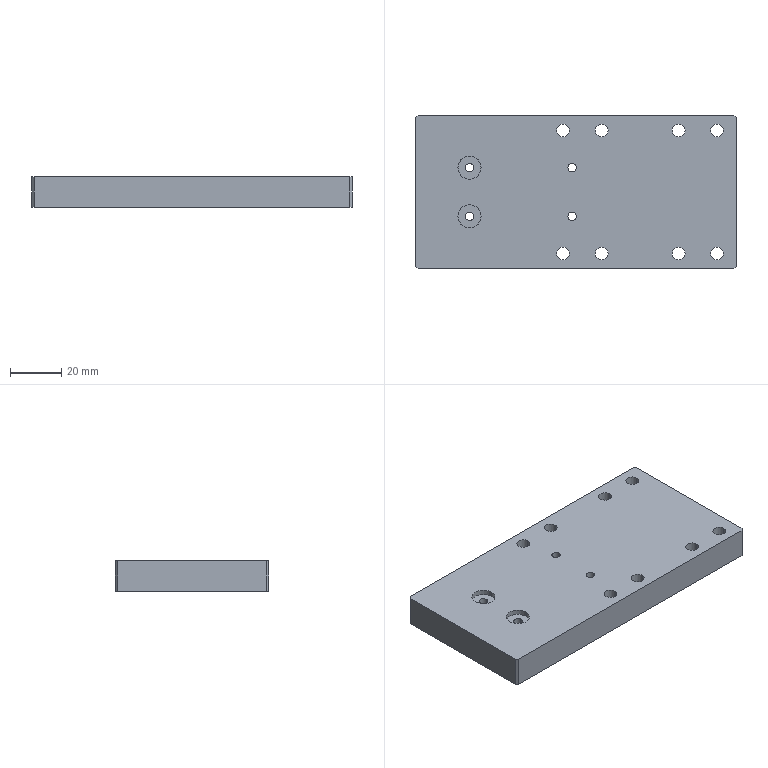Part | SolidWorks | features HoleWzd 3, Chamfer 1, Cut 1, Extrusion 1 | 1 solid | 40 faces | box 125 x 60 x 12 mm | volume 87460 mm3 | cylinder 28 | plane 12 | commonest cylinder face diameters 5 x16 3.3 x8 9 x4
STEP:
#1=CARTESIAN_POINT('',(7.5,24.,-6.));
#2=VERTEX_POINT('',#1);
#3=CARTESIAN_POINT('',(12.5,24.,-6.));
#4=VERTEX_POINT('',#3);
#5=CARTESIAN_POINT('',(10.,24.,-6.));
#6=DIRECTION('',(0.,0.,1.));
#7=DIRECTION('',(1.,0.,0.));
#8=AXIS2_PLACEMENT_3D('',#5,#6,#7);
#9=CIRCLE('',#8,2.5);
#10=EDGE_CURVE('',#2,#4,#9,.T.);
#11=ORIENTED_EDGE('',*,*,#10,.F.);
#12=CARTESIAN_POINT('',(7.5,24.,6.));
#13=VERTEX_POINT('',#12);
#14=CARTESIAN_POINT('',(7.5,24.,6.));
#15=DIRECTION('',(0.,0.,1.));
#16=VECTOR('',#15,1000.);
#17=LINE('',#14,#16);
#18=EDGE_CURVE('',#2,#13,#17,.T.);
#19=ORIENTED_EDGE('',*,*,#18,.T.);
#20=CARTESIAN_POINT('',(12.5,24.,6.));
#21=VERTEX_POINT('',#20);
#22=CARTESIAN_POINT('',(10.,24.,6.));
#23=DIRECTION('',(0.,0.,1.));
#24=DIRECTION('',(1.,0.,0.));
#25=AXIS2_PLACEMENT_3D('',#22,#23,#24);
#26=CIRCLE('',#25,2.5);
#27=EDGE_CURVE('',#13,#21,#26,.T.);
#28=ORIENTED_EDGE('',*,*,#27,.T.);
#29=CARTESIAN_POINT('',(12.5,24.,6.));
#30=DIRECTION('',(0.,0.,1.));
#31=VECTOR('',#30,1000.);
#32=LINE('',#29,#31);
#33=EDGE_CURVE('',#4,#21,#32,.T.);
#34=ORIENTED_EDGE('',*,*,#33,.F.);
#35=EDGE_LOOP('',(#11,#19,#28,#34));
#36=FACE_OUTER_BOUND('',#35,.T.);
#37=CARTESIAN_POINT('',(10.,24.,6.));
#38=DIRECTION('',(0.,0.,1.));
#39=DIRECTION('',(1.,0.,0.));
#40=AXIS2_PLACEMENT_3D('',#37,#38,#39);
#41=CYLINDRICAL_SURFACE('',#40,2.5);
#42=ADVANCED_FACE('',(#36),#41,.F.);
#43=CARTESIAN_POINT('',(37.5,24.,-6.));
#44=VERTEX_POINT('',#43);
#45=CARTESIAN_POINT('',(42.5,24.,-6.));
#46=VERTEX_POINT('',#45);
#47=CARTESIAN_POINT('',(40.,24.,-6.));
#48=DIRECTION('',(0.,0.,1.));
#49=DIRECTION('',(1.,0.,0.));
#50=AXIS2_PLACEMENT_3D('',#47,#48,#49);
#51=CIRCLE('',#50,2.5);
#52=EDGE_CURVE('',#44,#46,#51,.T.);
#53=ORIENTED_EDGE('',*,*,#52,.F.);
#54=CARTESIAN_POINT('',(37.5,24.,6.));
#55=VERTEX_POINT('',#54);
#56=CARTESIAN_POINT('',(37.5,24.,6.));
#57=DIRECTION('',(0.,0.,1.));
#58=VECTOR('',#57,1000.);
#59=LINE('',#56,#58);
#60=EDGE_CURVE('',#44,#55,#59,.T.);
#61=ORIENTED_EDGE('',*,*,#60,.T.);
#62=CARTESIAN_POINT('',(42.5,24.,6.));
#63=VERTEX_POINT('',#62);
#64=CARTESIAN_POINT('',(40.,24.,6.));
#65=DIRECTION('',(0.,0.,1.));
#66=DIRECTION('',(1.,0.,0.));
#67=AXIS2_PLACEMENT_3D('',#64,#65,#66);
#68=CIRCLE('',#67,2.5);
#69=EDGE_CURVE('',#55,#63,#68,.T.);
#70=ORIENTED_EDGE('',*,*,#69,.T.);
#71=CARTESIAN_POINT('',(42.5,24.,6.));
#72=DIRECTION('',(0.,0.,1.));
#73=VECTOR('',#72,1000.);
#74=LINE('',#71,#73);
#75=EDGE_CURVE('',#46,#63,#74,.T.);
#76=ORIENTED_EDGE('',*,*,#75,.F.);
#77=EDGE_LOOP('',(#53,#61,#70,#76));
#78=FACE_OUTER_BOUND('',#77,.T.);
#79=CARTESIAN_POINT('',(40.,24.,6.));
#80=DIRECTION('',(0.,0.,1.));
#81=DIRECTION('',(1.,0.,0.));
#82=AXIS2_PLACEMENT_3D('',#79,#80,#81);
#83=CYLINDRICAL_SURFACE('',#82,2.5);
#84=ADVANCED_FACE('',(#78),#83,.F.);
#85=CARTESIAN_POINT('',(7.5,-24.,-6.));
#86=VERTEX_POINT('',#85);
#87=CARTESIAN_POINT('',(12.5,-24.,-6.));
#88=VERTEX_POINT('',#87);
#89=CARTESIAN_POINT('',(10.,-24.,-6.));
#90=DIRECTION('',(0.,0.,1.));
#91=DIRECTION('',(1.,0.,0.));
#92=AXIS2_PLACEMENT_3D('',#89,#90,#91);
#93=CIRCLE('',#92,2.5);
#94=EDGE_CURVE('',#86,#88,#93,.T.);
#95=ORIENTED_EDGE('',*,*,#94,.F.);
#96=CARTESIAN_POINT('',(7.5,-24.,6.));
#97=VERTEX_POINT('',#96);
#98=CARTESIAN_POINT('',(7.5,-24.,6.));
#99=DIRECTION('',(0.,0.,1.));
#100=VECTOR('',#99,1000.);
#101=LINE('',#98,#100);
#102=EDGE_CURVE('',#86,#97,#101,.T.);
#103=ORIENTED_EDGE('',*,*,#102,.T.);
#104=CARTESIAN_POINT('',(12.5,-24.,6.));
#105=VERTEX_POINT('',#104);
#106=CARTESIAN_POINT('',(10.,-24.,6.));
#107=DIRECTION('',(0.,0.,1.));
#108=DIRECTION('',(1.,0.,0.));
#109=AXIS2_PLACEMENT_3D('',#106,#107,#108);
#110=CIRCLE('',#109,2.5);
#111=EDGE_CURVE('',#97,#105,#110,.T.);
#112=ORIENTED_EDGE('',*,*,#111,.T.);
#113=CARTESIAN_POINT('',(12.5,-24.,6.));
#114=DIRECTION('',(0.,0.,1.));
#115=VECTOR('',#114,1000.);
#116=LINE('',#113,#115);
#117=EDGE_CURVE('',#88,#105,#116,.T.);
#118=ORIENTED_EDGE('',*,*,#117,.F.);
#119=EDGE_LOOP('',(#95,#103,#112,#118));
#120=FACE_OUTER_BOUND('',#119,.T.);
#121=CARTESIAN_POINT('',(10.,-24.,6.));
#122=DIRECTION('',(0.,0.,1.));
#123=DIRECTION('',(1.,0.,0.));
#124=AXIS2_PLACEMENT_3D('',#121,#122,#123);
#125=CYLINDRICAL_SURFACE('',#124,2.5);
#126=ADVANCED_FACE('',(#120),#125,.F.);
#127=CARTESIAN_POINT('',(37.5,-24.,-6.));
#128=VERTEX_POINT('',#127);
#129=CARTESIAN_POINT('',(42.5,-24.,-6.));
#130=VERTEX_POINT('',#129);
#131=CARTESIAN_POINT('',(40.,-24.,-6.));
#132=DIRECTION('',(0.,0.,1.));
#133=DIRECTION('',(1.,0.,0.));
#134=AXIS2_PLACEMENT_3D('',#131,#132,#133);
#135=CIRCLE('',#134,2.5);
#136=EDGE_CURVE('',#128,#130,#135,.T.);
#137=ORIENTED_EDGE('',*,*,#136,.F.);
#138=CARTESIAN_POINT('',(37.5,-24.,6.));
#139=VERTEX_POINT('',#138);
#140=CARTESIAN_POINT('',(37.5,-24.,6.));
#141=DIRECTION('',(0.,0.,1.));
#142=VECTOR('',#141,1000.);
#143=LINE('',#140,#142);
#144=EDGE_CURVE('',#128,#139,#143,.T.);
#145=ORIENTED_EDGE('',*,*,#144,.T.);
#146=CARTESIAN_POINT('',(42.5,-24.,6.));
#147=VERTEX_POINT('',#146);
#148=CARTESIAN_POINT('',(40.,-24.,6.));
#149=DIRECTION('',(0.,0.,1.));
#150=DIRECTION('',(1.,0.,0.));
#151=AXIS2_PLACEMENT_3D('',#148,#149,#150);
#152=CIRCLE('',#151,2.5);
#153=EDGE_CURVE('',#139,#147,#152,.T.);
#154=ORIENTED_EDGE('',*,*,#153,.T.);
#155=CARTESIAN_POINT('',(42.5,-24.,6.));
#156=DIRECTION('',(0.,0.,1.));
#157=VECTOR('',#156,1000.);
#158=LINE('',#155,#157);
#159=EDGE_CURVE('',#130,#147,#158,.T.);
#160=ORIENTED_EDGE('',*,*,#159,.F.);
#161=EDGE_LOOP('',(#137,#145,#154,#160));
#162=FACE_OUTER_BOUND('',#161,.T.);
#163=CARTESIAN_POINT('',(40.,-24.,6.));
#164=DIRECTION('',(0.,0.,1.));
#165=DIRECTION('',(1.,0.,0.));
#166=AXIS2_PLACEMENT_3D('',#163,#164,#165);
#167=CYLINDRICAL_SURFACE('',#166,2.5);
#168=ADVANCED_FACE('',(#162),#167,.F.);
#169=CARTESIAN_POINT('',(-46.,9.5,4.));
#170=VERTEX_POINT('',#169);
#171=CARTESIAN_POINT('',(-37.,9.5,4.));
#172=VERTEX_POINT('',#171);
#173=CARTESIAN_POINT('',(-41.5,9.5,4.));
#174=DIRECTION('',(0.,0.,1.));
#175=DIRECTION('',(1.,0.,0.));
#176=AXIS2_PLACEMENT_3D('',#173,#174,#175);
#177=CIRCLE('',#176,4.5);
#178=EDGE_CURVE('',#170,#172,#177,.T.);
#179=ORIENTED_EDGE('',*,*,#178,.F.);
#180=CARTESIAN_POINT('',(-46.,9.5,6.));
#181=VERTEX_POINT('',#180);
#182=CARTESIAN_POINT('',(-46.,9.5,4.));
#183=DIRECTION('',(0.,0.,1.));
#184=VECTOR('',#183,1000.);
#185=LINE('',#182,#184);
#186=EDGE_CURVE('',#170,#181,#185,.T.);
#187=ORIENTED_EDGE('',*,*,#186,.T.);
#188=CARTESIAN_POINT('',(-37.,9.5,6.));
#189=VERTEX_POINT('',#188);
#190=CARTESIAN_POINT('',(-41.5,9.5,6.));
#191=DIRECTION('',(0.,0.,1.));
#192=DIRECTION('',(1.,0.,0.));
#193=AXIS2_PLACEMENT_3D('',#190,#191,#192);
#194=CIRCLE('',#193,4.5);
#195=EDGE_CURVE('',#181,#189,#194,.T.);
#196=ORIENTED_EDGE('',*,*,#195,.T.);
#197=CARTESIAN_POINT('',(-37.,9.5,4.));
#198=DIRECTION('',(0.,0.,1.));
#199=VECTOR('',#198,1000.);
#200=LINE('',#197,#199);
#201=EDGE_CURVE('',#172,#189,#200,.T.);
#202=ORIENTED_EDGE('',*,*,#201,.F.);
#203=EDGE_LOOP('',(#179,#187,#196,#202));
#204=FACE_OUTER_BOUND('',#203,.T.);
#205=CARTESIAN_POINT('',(-41.5,9.5,4.));
#206=DIRECTION('',(0.,0.,1.));
#207=DIRECTION('',(1.,0.,0.));
#208=AXIS2_PLACEMENT_3D('',#205,#206,#207);
#209=CYLINDRICAL_SURFACE('',#208,4.5);
#210=ADVANCED_FACE('',(#204),#209,.F.);
#211=CARTESIAN_POINT('',(-46.,-9.5,4.));
#212=VERTEX_POINT('',#211);
#213=CARTESIAN_POINT('',(-37.,-9.5,4.));
#214=VERTEX_POINT('',#213);
#215=CARTESIAN_POINT('',(-41.5,-9.5,4.));
#216=DIRECTION('',(0.,0.,1.));
#217=DIRECTION('',(1.,0.,0.));
#218=AXIS2_PLACEMENT_3D('',#215,#216,#217);
#219=CIRCLE('',#218,4.5);
#220=EDGE_CURVE('',#212,#214,#219,.T.);
#221=ORIENTED_EDGE('',*,*,#220,.F.);
#222=CARTESIAN_POINT('',(-46.,-9.5,6.));
#223=VERTEX_POINT('',#222);
#224=CARTESIAN_POINT('',(-46.,-9.5,4.));
#225=DIRECTION('',(0.,0.,1.));
#226=VECTOR('',#225,1000.);
#227=LINE('',#224,#226);
#228=EDGE_CURVE('',#212,#223,#227,.T.);
#229=ORIENTED_EDGE('',*,*,#228,.T.);
#230=CARTESIAN_POINT('',(-37.,-9.5,6.));
#231=VERTEX_POINT('',#230);
#232=CARTESIAN_POINT('',(-41.5,-9.5,6.));
#233=DIRECTION('',(0.,0.,1.));
#234=DIRECTION('',(1.,0.,0.));
#235=AXIS2_PLACEMENT_3D('',#232,#233,#234);
#236=CIRCLE('',#235,4.5);
#237=EDGE_CURVE('',#223,#231,#236,.T.);
#238=ORIENTED_EDGE('',*,*,#237,.T.);
#239=CARTESIAN_POINT('',(-37.,-9.5,4.));
#240=DIRECTION('',(0.,0.,1.));
#241=VECTOR('',#240,1000.);
#242=LINE('',#239,#241);
#243=EDGE_CURVE('',#214,#231,#242,.T.);
#244=ORIENTED_EDGE('',*,*,#243,.F.);
#245=EDGE_LOOP('',(#221,#229,#238,#244));
#246=FACE_OUTER_BOUND('',#245,.T.);
#247=CARTESIAN_POINT('',(-41.5,-9.5,4.));
#248=DIRECTION('',(0.,0.,1.));
#249=DIRECTION('',(1.,0.,0.));
#250=AXIS2_PLACEMENT_3D('',#247,#248,#249);
#251=CYLINDRICAL_SURFACE('',#250,4.5);
#252=ADVANCED_FACE('',(#246),#251,.F.);
#253=CARTESIAN_POINT('',(-3.15,9.5,-6.));
#254=VERTEX_POINT('',#253);
#255=CARTESIAN_POINT('',(0.15,9.5,-6.));
#256=VERTEX_POINT('',#255);
#257=CARTESIAN_POINT('',(-1.5,9.5,-6.));
#258=DIRECTION('',(0.,0.,1.));
#259=DIRECTION('',(1.,0.,0.));
#260=AXIS2_PLACEMENT_3D('',#257,#258,#259);
#261=CIRCLE('',#260,1.65);
#262=EDGE_CURVE('',#254,#256,#261,.T.);
#263=ORIENTED_EDGE('',*,*,#262,.F.);
#264=CARTESIAN_POINT('',(-3.15,9.5,6.));
#265=VERTEX_POINT('',#264);
#266=CARTESIAN_POINT('',(-3.15,9.5,6.));
#267=DIRECTION('',(0.,0.,1.));
#268=VECTOR('',#267,1000.);
#269=LINE('',#266,#268);
#270=EDGE_CURVE('',#254,#265,#269,.T.);
#271=ORIENTED_EDGE('',*,*,#270,.T.);
#272=CARTESIAN_POINT('',(0.15,9.5,6.));
#273=VERTEX_POINT('',#272);
#274=CARTESIAN_POINT('',(-1.5,9.5,6.));
#275=DIRECTION('',(0.,0.,1.));
#276=DIRECTION('',(1.,0.,0.));
#277=AXIS2_PLACEMENT_3D('',#274,#275,#276);
#278=CIRCLE('',#277,1.65);
#279=EDGE_CURVE('',#265,#273,#278,.T.);
#280=ORIENTED_EDGE('',*,*,#279,.T.);
#281=CARTESIAN_POINT('',(0.15,9.5,6.));
#282=DIRECTION('',(0.,0.,1.));
#283=VECTOR('',#282,1000.);
#284=LINE('',#281,#283);
#285=EDGE_CURVE('',#256,#273,#284,.T.);
#286=ORIENTED_EDGE('',*,*,#285,.F.);
#287=EDGE_LOOP('',(#263,#271,#280,#286));
#288=FACE_OUTER_BOUND('',#287,.T.);
#289=CARTESIAN_POINT('',(-1.5,9.5,6.));
#290=DIRECTION('',(0.,0.,1.));
#291=DIRECTION('',(1.,0.,0.));
#292=AXIS2_PLACEMENT_3D('',#289,#290,#291);
#293=CYLINDRICAL_SURFACE('',#292,1.65);
#294=ADVANCED_FACE('',(#288),#293,.F.);
#295=CARTESIAN_POINT('',(-3.15,-9.5,-6.));
#296=VERTEX_POINT('',#295);
#297=CARTESIAN_POINT('',(0.15,-9.5,-6.));
#298=VERTEX_POINT('',#297);
#299=CARTESIAN_POINT('',(-1.5,-9.5,-6.));
#300=DIRECTION('',(0.,0.,1.));
#301=DIRECTION('',(1.,0.,0.));
#302=AXIS2_PLACEMENT_3D('',#299,#300,#301);
#303=CIRCLE('',#302,1.65);
#304=EDGE_CURVE('',#296,#298,#303,.T.);
#305=ORIENTED_EDGE('',*,*,#304,.F.);
#306=CARTESIAN_POINT('',(-3.15,-9.5,6.));
#307=VERTEX_POINT('',#306);
#308=CARTESIAN_POINT('',(-3.15,-9.5,6.));
#309=DIRECTION('',(0.,0.,1.));
#310=VECTOR('',#309,1000.);
#311=LINE('',#308,#310);
#312=EDGE_CURVE('',#296,#307,#311,.T.);
#313=ORIENTED_EDGE('',*,*,#312,.T.);
#314=CARTESIAN_POINT('',(0.15,-9.5,6.));
#315=VERTEX_POINT('',#314);
#316=CARTESIAN_POINT('',(-1.5,-9.5,6.));
#317=DIRECTION('',(0.,0.,1.));
#318=DIRECTION('',(1.,0.,0.));
#319=AXIS2_PLACEMENT_3D('',#316,#317,#318);
#320=CIRCLE('',#319,1.65);
#321=EDGE_CURVE('',#307,#315,#320,.T.);
#322=ORIENTED_EDGE('',*,*,#321,.T.);
#323=CARTESIAN_POINT('',(0.15,-9.5,6.));
#324=DIRECTION('',(0.,0.,1.));
#325=VECTOR('',#324,1000.);
#326=LINE('',#323,#325);
#327=EDGE_CURVE('',#298,#315,#326,.T.);
#328=ORIENTED_EDGE('',*,*,#327,.F.);
#329=EDGE_LOOP('',(#305,#313,#322,#328));
#330=FACE_OUTER_BOUND('',#329,.T.);
#331=CARTESIAN_POINT('',(-1.5,-9.5,6.));
#332=DIRECTION('',(0.,0.,1.));
#333=DIRECTION('',(1.,0.,0.));
#334=AXIS2_PLACEMENT_3D('',#331,#332,#333);
#335=CYLINDRICAL_SURFACE('',#334,1.65);
#336=ADVANCED_FACE('',(#330),#335,.F.);
#337=CARTESIAN_POINT('',(-2.5,24.,6.));
#338=VERTEX_POINT('',#337);
#339=CARTESIAN_POINT('',(-7.5,24.,6.));
#340=VERTEX_POINT('',#339);
#341=CARTESIAN_POINT('',(-5.,24.,6.));
#342=DIRECTION('',(0.,0.,-1.));
#343=DIRECTION('',(-1.,0.,0.));
#344=AXIS2_PLACEMENT_3D('',#341,#342,#343);
#345=CIRCLE('',#344,2.5);
#346=EDGE_CURVE('',#338,#340,#345,.T.);
#347=ORIENTED_EDGE('',*,*,#346,.F.);
#348=CARTESIAN_POINT('',(-2.5,24.,-6.));
#349=VERTEX_POINT('',#348);
#350=CARTESIAN_POINT('',(-2.5,24.,-6.));
#351=DIRECTION('',(0.,0.,-1.));
#352=VECTOR('',#351,1000.);
#353=LINE('',#350,#352);
#354=EDGE_CURVE('',#338,#349,#353,.T.);
#355=ORIENTED_EDGE('',*,*,#354,.T.);
#356=CARTESIAN_POINT('',(-7.5,24.,-6.));
#357=VERTEX_POINT('',#356);
#358=CARTESIAN_POINT('',(-5.,24.,-6.));
#359=DIRECTION('',(0.,0.,-1.));
#360=DIRECTION('',(-1.,0.,0.));
#361=AXIS2_PLACEMENT_3D('',#358,#359,#360);
#362=CIRCLE('',#361,2.5);
#363=EDGE_CURVE('',#349,#357,#362,.T.);
#364=ORIENTED_EDGE('',*,*,#363,.T.);
#365=CARTESIAN_POINT('',(-7.5,24.,-6.));
#366=DIRECTION('',(0.,0.,-1.));
#367=VECTOR('',#366,1000.);
#368=LINE('',#365,#367);
#369=EDGE_CURVE('',#340,#357,#368,.T.);
#370=ORIENTED_EDGE('',*,*,#369,.F.);
#371=EDGE_LOOP('',(#347,#355,#364,#370));
#372=FACE_OUTER_BOUND('',#371,.T.);
#373=CARTESIAN_POINT('',(-5.,24.,-6.));
#374=DIRECTION('',(0.,0.,-1.));
#375=DIRECTION('',(-1.,0.,0.));
#376=AXIS2_PLACEMENT_3D('',#373,#374,#375);
#377=CYLINDRICAL_SURFACE('',#376,2.5);
#378=ADVANCED_FACE('',(#372),#377,.F.);
#379=CARTESIAN_POINT('',(-2.5,-24.,6.));
#380=VERTEX_POINT('',#379);
#381=CARTESIAN_POINT('',(-7.5,-24.,6.));
#382=VERTEX_POINT('',#381);
#383=CARTESIAN_POINT('',(-5.,-24.,6.));
#384=DIRECTION('',(0.,0.,-1.));
#385=DIRECTION('',(-1.,0.,0.));
#386=AXIS2_PLACEMENT_3D('',#383,#384,#385);
#387=CIRCLE('',#386,2.5);
#388=EDGE_CURVE('',#380,#382,#387,.T.);
#389=ORIENTED_EDGE('',*,*,#388,.F.);
#390=CARTESIAN_POINT('',(-2.5,-24.,-6.));
#391=VERTEX_POINT('',#390);
#392=CARTESIAN_POINT('',(-2.5,-24.,-6.));
#393=DIRECTION('',(0.,0.,-1.));
#394=VECTOR('',#393,1000.);
#395=LINE('',#392,#394);
#396=EDGE_CURVE('',#380,#391,#395,.T.);
#397=ORIENTED_EDGE('',*,*,#396,.T.);
#398=CARTESIAN_POINT('',(-7.5,-24.,-6.));
#399=VERTEX_POINT('',#398);
#400=CARTESIAN_POINT('',(-5.,-24.,-6.));
#401=DIRECTION('',(0.,0.,-1.));
#402=DIRECTION('',(-1.,0.,0.));
#403=AXIS2_PLACEMENT_3D('',#400,#401,#402);
#404=CIRCLE('',#403,2.5);
#405=EDGE_CURVE('',#391,#399,#404,.T.);
#406=ORIENTED_EDGE('',*,*,#405,.T.);
#407=CARTESIAN_POINT('',(-7.5,-24.,-6.));
#408=DIRECTION('',(0.,0.,-1.));
#409=VECTOR('',#408,1000.);
#410=LINE('',#407,#409);
#411=EDGE_CURVE('',#382,#399,#410,.T.);
#412=ORIENTED_EDGE('',*,*,#411,.F.);
#413=EDGE_LOOP('',(#389,#397,#406,#412));
#414=FACE_OUTER_BOUND('',#413,.T.);
#415=CARTESIAN_POINT('',(-5.,-24.,-6.));
#416=DIRECTION('',(0.,0.,-1.));
#417=DIRECTION('',(-1.,0.,0.));
#418=AXIS2_PLACEMENT_3D('',#415,#416,#417);
#419=CYLINDRICAL_SURFACE('',#418,2.5);
#420=ADVANCED_FACE('',(#414),#419,.F.);
#421=CARTESIAN_POINT('',(57.5,-24.,6.));
#422=VERTEX_POINT('',#421);
#423=CARTESIAN_POINT('',(52.5,-24.,6.));
#424=VERTEX_POINT('',#423);
#425=CARTESIAN_POINT('',(55.,-24.,6.));
#426=DIRECTION('',(0.,0.,-1.));
#427=DIRECTION('',(-1.,0.,0.));
#428=AXIS2_PLACEMENT_3D('',#425,#426,#427);
#429=CIRCLE('',#428,2.5);
#430=EDGE_CURVE('',#422,#424,#429,.T.);
#431=ORIENTED_EDGE('',*,*,#430,.F.);
#432=CARTESIAN_POINT('',(57.5,-24.,-6.));
#433=VERTEX_POINT('',#432);
#434=CARTESIAN_POINT('',(57.5,-24.,-6.));
#435=DIRECTION('',(0.,0.,-1.));
#436=VECTOR('',#435,1000.);
#437=LINE('',#434,#436);
#438=EDGE_CURVE('',#422,#433,#437,.T.);
#439=ORIENTED_EDGE('',*,*,#438,.T.);
#440=CARTESIAN_POINT('',(52.5,-24.,-6.));
#441=VERTEX_POINT('',#440);
#442=CARTESIAN_POINT('',(55.,-24.,-6.));
#443=DIRECTION('',(0.,0.,-1.));
#444=DIRECTION('',(-1.,0.,0.));
#445=AXIS2_PLACEMENT_3D('',#442,#443,#444);
#446=CIRCLE('',#445,2.5);
#447=EDGE_CURVE('',#433,#441,#446,.T.);
#448=ORIENTED_EDGE('',*,*,#447,.T.);
#449=CARTESIAN_POINT('',(52.5,-24.,-6.));
#450=DIRECTION('',(0.,0.,-1.));
#451=VECTOR('',#450,1000.);
#452=LINE('',#449,#451);
#453=EDGE_CURVE('',#424,#441,#452,.T.);
#454=ORIENTED_EDGE('',*,*,#453,.F.);
#455=EDGE_LOOP('',(#431,#439,#448,#454));
#456=FACE_OUTER_BOUND('',#455,.T.);
#457=CARTESIAN_POINT('',(55.,-24.,-6.));
#458=DIRECTION('',(0.,0.,-1.));
#459=DIRECTION('',(-1.,0.,0.));
#460=AXIS2_PLACEMENT_3D('',#457,#458,#459);
#461=CYLINDRICAL_SURFACE('',#460,2.5);
#462=ADVANCED_FACE('',(#456),#461,.F.);
#463=CARTESIAN_POINT('',(57.5,24.,6.));
#464=VERTEX_POINT('',#463);
#465=CARTESIAN_POINT('',(52.5,24.,6.));
#466=VERTEX_POINT('',#465);
#467=CARTESIAN_POINT('',(55.,24.,6.));
#468=DIRECTION('',(0.,0.,-1.));
#469=DIRECTION('',(-1.,0.,0.));
#470=AXIS2_PLACEMENT_3D('',#467,#468,#469);
#471=CIRCLE('',#470,2.5);
#472=EDGE_CURVE('',#464,#466,#471,.T.);
#473=ORIENTED_EDGE('',*,*,#472,.F.);
#474=CARTESIAN_POINT('',(57.5,24.,-6.));
#475=VERTEX_POINT('',#474);
#476=CARTESIAN_POINT('',(57.5,24.,-6.));
#477=DIRECTION('',(0.,0.,-1.));
#478=VECTOR('',#477,1000.);
#479=LINE('',#476,#478);
#480=EDGE_CURVE('',#464,#475,#479,.T.);
#481=ORIENTED_EDGE('',*,*,#480,.T.);
#482=CARTESIAN_POINT('',(52.5,24.,-6.));
#483=VERTEX_POINT('',#482);
#484=CARTESIAN_POINT('',(55.,24.,-6.));
#485=DIRECTION('',(0.,0.,-1.));
#486=DIRECTION('',(-1.,0.,0.));
#487=AXIS2_PLACEMENT_3D('',#484,#485,#486);
#488=CIRCLE('',#487,2.5);
#489=EDGE_CURVE('',#475,#483,#488,.T.);
#490=ORIENTED_EDGE('',*,*,#489,.T.);
#491=CARTESIAN_POINT('',(52.5,24.,-6.));
#492=DIRECTION('',(0.,0.,-1.));
#493=VECTOR('',#492,1000.);
#494=LINE('',#491,#493);
#495=EDGE_CURVE('',#466,#483,#494,.T.);
#496=ORIENTED_EDGE('',*,*,#495,.F.);
#497=EDGE_LOOP('',(#473,#481,#490,#496));
#498=FACE_OUTER_BOUND('',#497,.T.);
#499=CARTESIAN_POINT('',(55.,24.,-6.));
#500=DIRECTION('',(0.,0.,-1.));
#501=DIRECTION('',(-1.,0.,0.));
#502=AXIS2_PLACEMENT_3D('',#499,#500,#501);
#503=CYLINDRICAL_SURFACE('',#502,2.5);
#504=ADVANCED_FACE('',(#498),#503,.F.);
#505=CARTESIAN_POINT('',(-43.15,-9.5,-6.));
#506=VERTEX_POINT('',#505);
#507=CARTESIAN_POINT('',(-39.85,-9.5,-6.));
#508=VERTEX_POINT('',#507);
#509=CARTESIAN_POINT('',(-41.5,-9.5,-6.));
#510=DIRECTION('',(0.,0.,1.));
#511=DIRECTION('',(1.,0.,0.));
#512=AXIS2_PLACEMENT_3D('',#509,#510,#511);
#513=CIRCLE('',#512,1.65);
#514=EDGE_CURVE('',#506,#508,#513,.T.);
#515=ORIENTED_EDGE('',*,*,#514,.F.);
#516=CARTESIAN_POINT('',(-43.15,-9.5,4.));
#517=VERTEX_POINT('',#516);
#518=CARTESIAN_POINT('',(-43.15,-9.5,6.));
#519=DIRECTION('',(0.,0.,1.));
#520=VECTOR('',#519,1000.);
#521=LINE('',#518,#520);
#522=EDGE_CURVE('',#506,#517,#521,.T.);
#523=ORIENTED_EDGE('',*,*,#522,.T.);
#524=CARTESIAN_POINT('',(-39.85,-9.5,4.));
#525=VERTEX_POINT('',#524);
#526=CARTESIAN_POINT('',(-41.5,-9.5,4.));
#527=DIRECTION('',(0.,0.,-1.));
#528=DIRECTION('',(1.,0.,0.));
#529=AXIS2_PLACEMENT_3D('',#526,#527,#528);
#530=CIRCLE('',#529,1.65);
#531=EDGE_CURVE('',#525,#517,#530,.T.);
#532=ORIENTED_EDGE('',*,*,#531,.F.);
#533=CARTESIAN_POINT('',(-39.85,-9.5,6.));
#534=DIRECTION('',(0.,0.,1.));
#535=VECTOR('',#534,1000.);
#536=LINE('',#533,#535);
#537=EDGE_CURVE('',#508,#525,#536,.T.);
#538=ORIENTED_EDGE('',*,*,#537,.F.);
#539=EDGE_LOOP('',(#515,#523,#532,#538));
#540=FACE_OUTER_BOUND('',#539,.T.);
#541=CARTESIAN_POINT('',(-41.5,-9.5,6.));
#542=DIRECTION('',(0.,0.,1.));
#543=DIRECTION('',(1.,0.,0.));
#544=AXIS2_PLACEMENT_3D('',#541,#542,#543);
#545=CYLINDRICAL_SURFACE('',#544,1.65);
#546=ADVANCED_FACE('',(#540),#545,.F.);
#547=CARTESIAN_POINT('',(-43.15,9.5,-6.));
#548=VERTEX_POINT('',#547);
#549=CARTESIAN_POINT('',(-39.85,9.5,-6.));
#550=VERTEX_POINT('',#549);
#551=CARTESIAN_POINT('',(-41.5,9.5,-6.));
#552=DIRECTION('',(0.,0.,1.));
#553=DIRECTION('',(1.,0.,0.));
#554=AXIS2_PLACEMENT_3D('',#551,#552,#553);
#555=CIRCLE('',#554,1.65);
#556=EDGE_CURVE('',#548,#550,#555,.T.);
#557=ORIENTED_EDGE('',*,*,#556,.F.);
#558=CARTESIAN_POINT('',(-43.15,9.5,4.));
#559=VERTEX_POINT('',#558);
#560=CARTESIAN_POINT('',(-43.15,9.5,6.));
#561=DIRECTION('',(0.,0.,1.));
#562=VECTOR('',#561,1000.);
#563=LINE('',#560,#562);
#564=EDGE_CURVE('',#548,#559,#563,.T.);
#565=ORIENTED_EDGE('',*,*,#564,.T.);
#566=CARTESIAN_POINT('',(-39.85,9.5,4.));
#567=VERTEX_POINT('',#566);
#568=CARTESIAN_POINT('',(-41.5,9.5,4.));
#569=DIRECTION('',(0.,0.,-1.));
#570=DIRECTION('',(1.,0.,0.));
#571=AXIS2_PLACEMENT_3D('',#568,#569,#570);
#572=CIRCLE('',#571,1.65);
#573=EDGE_CURVE('',#567,#559,#572,.T.);
#574=ORIENTED_EDGE('',*,*,#573,.F.);
#575=CARTESIAN_POINT('',(-39.85,9.5,6.));
#576=DIRECTION('',(0.,0.,1.));
#577=VECTOR('',#576,1000.);
#578=LINE('',#575,#577);
#579=EDGE_CURVE('',#550,#567,#578,.T.);
#580=ORIENTED_EDGE('',*,*,#579,.F.);
#581=EDGE_LOOP('',(#557,#565,#574,#580));
#582=FACE_OUTER_BOUND('',#581,.T.);
#583=CARTESIAN_POINT('',(-41.5,9.5,6.));
#584=DIRECTION('',(0.,0.,1.));
#585=DIRECTION('',(1.,0.,0.));
#586=AXIS2_PLACEMENT_3D('',#583,#584,#585);
#587=CYLINDRICAL_SURFACE('',#586,1.65);
#588=ADVANCED_FACE('',(#582),#587,.F.);
#589=ORIENTED_EDGE('',*,*,#564,.F.);
#590=CARTESIAN_POINT('',(-41.5,9.5,-6.));
#591=DIRECTION('',(0.,0.,1.));
#592=DIRECTION('',(1.,0.,0.));
#593=AXIS2_PLACEMENT_3D('',#590,#591,#592);
#594=CIRCLE('',#593,1.65);
#595=EDGE_CURVE('',#550,#548,#594,.T.);
#596=ORIENTED_EDGE('',*,*,#595,.F.);
#597=ORIENTED_EDGE('',*,*,#579,.T.);
#598=CARTESIAN_POINT('',(-41.5,9.5,4.));
#599=DIRECTION('',(0.,0.,-1.));
#600=DIRECTION('',(1.,0.,0.));
#601=AXIS2_PLACEMENT_3D('',#598,#599,#600);
#602=CIRCLE('',#601,1.65);
#603=EDGE_CURVE('',#559,#567,#602,.T.);
#604=ORIENTED_EDGE('',*,*,#603,.F.);
#605=EDGE_LOOP('',(#589,#596,#597,#604));
#606=FACE_OUTER_BOUND('',#605,.T.);
#607=CARTESIAN_POINT('',(-41.5,9.5,6.));
#608=DIRECTION('',(0.,0.,1.));
#609=DIRECTION('',(1.,0.,0.));
#610=AXIS2_PLACEMENT_3D('',#607,#608,#609);
#611=CYLINDRICAL_SURFACE('',#610,1.65);
#612=ADVANCED_FACE('',(#606),#611,.F.);
#613=ORIENTED_EDGE('',*,*,#522,.F.);
#614=CARTESIAN_POINT('',(-41.5,-9.5,-6.));
#615=DIRECTION('',(0.,0.,1.));
#616=DIRECTION('',(1.,0.,0.));
#617=AXIS2_PLACEMENT_3D('',#614,#615,#616);
#618=CIRCLE('',#617,1.65);
#619=EDGE_CURVE('',#508,#506,#618,.T.);
#620=ORIENTED_EDGE('',*,*,#619,.F.);
#621=ORIENTED_EDGE('',*,*,#537,.T.);
#622=CARTESIAN_POINT('',(-41.5,-9.5,4.));
#623=DIRECTION('',(0.,0.,-1.));
#624=DIRECTION('',(1.,0.,0.));
#625=AXIS2_PLACEMENT_3D('',#622,#623,#624);
#626=CIRCLE('',#625,1.65);
#627=EDGE_CURVE('',#517,#525,#626,.T.);
#628=ORIENTED_EDGE('',*,*,#627,.F.);
#629=EDGE_LOOP('',(#613,#620,#621,#628));
#630=FACE_OUTER_BOUND('',#629,.T.);
#631=CARTESIAN_POINT('',(-41.5,-9.5,6.));
#632=DIRECTION('',(0.,0.,1.));
#633=DIRECTION('',(1.,0.,0.));
#634=AXIS2_PLACEMENT_3D('',#631,#632,#633);
#635=CYLINDRICAL_SURFACE('',#634,1.65);
#636=ADVANCED_FACE('',(#630),#635,.F.);
#637=CARTESIAN_POINT('',(62.5,-29.,6.));
#638=VERTEX_POINT('',#637);
#639=CARTESIAN_POINT('',(62.5,29.,6.));
#640=VERTEX_POINT('',#639);
#641=CARTESIAN_POINT('',(62.5,30.,6.));
#642=DIRECTION('',(0.,1.,0.));
#643=VECTOR('',#642,1000.);
#644=LINE('',#641,#643);
#645=EDGE_CURVE('',#638,#640,#644,.T.);
#646=ORIENTED_EDGE('',*,*,#645,.F.);
#647=CARTESIAN_POINT('',(62.5,-29.,-6.));
#648=VERTEX_POINT('',#647);
#649=CARTESIAN_POINT('',(62.5,-29.,6.));
#650=DIRECTION('',(0.,0.,-1.));
#651=VECTOR('',#650,1000.);
#652=LINE('',#649,#651);
#653=EDGE_CURVE('',#638,#648,#652,.T.);
#654=ORIENTED_EDGE('',*,*,#653,.T.);
#655=CARTESIAN_POINT('',(62.5,29.,-6.));
#656=VERTEX_POINT('',#655);
#657=CARTESIAN_POINT('',(62.5,30.,-6.));
#658=DIRECTION('',(0.,1.,0.));
#659=VECTOR('',#658,1000.);
#660=LINE('',#657,#659);
#661=EDGE_CURVE('',#648,#656,#660,.T.);
#662=ORIENTED_EDGE('',*,*,#661,.T.);
#663=CARTESIAN_POINT('',(62.5,29.,6.));
#664=DIRECTION('',(0.,0.,1.));
#665=VECTOR('',#664,1000.);
#666=LINE('',#663,#665);
#667=EDGE_CURVE('',#656,#640,#666,.T.);
#668=ORIENTED_EDGE('',*,*,#667,.T.);
#669=EDGE_LOOP('',(#646,#654,#662,#668));
#670=FACE_OUTER_BOUND('',#669,.T.);
#671=CARTESIAN_POINT('',(62.5,30.,6.));
#672=DIRECTION('',(-1.,0.,0.));
#673=DIRECTION('',(0.,-1.,0.));
#674=AXIS2_PLACEMENT_3D('',#671,#672,#673);
#675=PLANE('',#674);
#676=ADVANCED_FACE('',(#670),#675,.F.);
#677=CARTESIAN_POINT('',(61.5,30.,6.));
#678=VERTEX_POINT('',#677);
#679=CARTESIAN_POINT('',(-61.5,30.,6.));
#680=VERTEX_POINT('',#679);
#681=CARTESIAN_POINT('',(-62.5,30.,6.));
#682=DIRECTION('',(-1.,0.,0.));
#683=VECTOR('',#682,1000.);
#684=LINE('',#681,#683);
#685=EDGE_CURVE('',#678,#680,#684,.T.);
#686=ORIENTED_EDGE('',*,*,#685,.F.);
#687=CARTESIAN_POINT('',(61.5,30.,-6.));
#688=VERTEX_POINT('',#687);
#689=CARTESIAN_POINT('',(61.5,30.,6.));
#690=DIRECTION('',(0.,0.,-1.));
#691=VECTOR('',#690,1000.);
#692=LINE('',#689,#691);
#693=EDGE_CURVE('',#678,#688,#692,.T.);
#694=ORIENTED_EDGE('',*,*,#693,.T.);
#695=CARTESIAN_POINT('',(-61.5,30.,-6.));
#696=VERTEX_POINT('',#695);
#697=CARTESIAN_POINT('',(-62.5,30.,-6.));
#698=DIRECTION('',(-1.,0.,0.));
#699=VECTOR('',#698,1000.);
#700=LINE('',#697,#699);
#701=EDGE_CURVE('',#688,#696,#700,.T.);
#702=ORIENTED_EDGE('',*,*,#701,.T.);
#703=CARTESIAN_POINT('',(-61.5,30.,6.));
#704=DIRECTION('',(0.,0.,1.));
#705=VECTOR('',#704,1000.);
#706=LINE('',#703,#705);
#707=EDGE_CURVE('',#696,#680,#706,.T.);
#708=ORIENTED_EDGE('',*,*,#707,.T.);
#709=EDGE_LOOP('',(#686,#694,#702,#708));
#710=FACE_OUTER_BOUND('',#709,.T.);
#711=CARTESIAN_POINT('',(-62.5,30.,6.));
#712=DIRECTION('',(0.,-1.,0.));
#713=DIRECTION('',(0.,0.,-1.));
#714=AXIS2_PLACEMENT_3D('',#711,#712,#713);
#715=PLANE('',#714);
#716=ADVANCED_FACE('',(#710),#715,.F.);
#717=CARTESIAN_POINT('',(-62.5,29.,6.));
#718=VERTEX_POINT('',#717);
#719=CARTESIAN_POINT('',(-62.5,-29.,6.));
#720=VERTEX_POINT('',#719);
#721=CARTESIAN_POINT('',(-62.5,30.,6.));
#722=DIRECTION('',(0.,-1.,0.));
#723=VECTOR('',#722,1000.);
#724=LINE('',#721,#723);
#725=EDGE_CURVE('',#718,#720,#724,.T.);
#726=ORIENTED_EDGE('',*,*,#725,.F.);
#727=CARTESIAN_POINT('',(-62.5,29.,-6.));
#728=VERTEX_POINT('',#727);
#729=CARTESIAN_POINT('',(-62.5,29.,6.));
#730=DIRECTION('',(0.,0.,-1.));
#731=VECTOR('',#730,1000.);
#732=LINE('',#729,#731);
#733=EDGE_CURVE('',#718,#728,#732,.T.);
#734=ORIENTED_EDGE('',*,*,#733,.T.);
#735=CARTESIAN_POINT('',(-62.5,-29.,-6.));
#736=VERTEX_POINT('',#735);
#737=CARTESIAN_POINT('',(-62.5,30.,-6.));
#738=DIRECTION('',(0.,-1.,0.));
#739=VECTOR('',#738,1000.);
#740=LINE('',#737,#739);
#741=EDGE_CURVE('',#728,#736,#740,.T.);
#742=ORIENTED_EDGE('',*,*,#741,.T.);
#743=CARTESIAN_POINT('',(-62.5,-29.,6.));
#744=DIRECTION('',(0.,0.,1.));
#745=VECTOR('',#744,1000.);
#746=LINE('',#743,#745);
#747=EDGE_CURVE('',#736,#720,#746,.T.);
#748=ORIENTED_EDGE('',*,*,#747,.T.);
#749=EDGE_LOOP('',(#726,#734,#742,#748));
#750=FACE_OUTER_BOUND('',#749,.T.);
#751=CARTESIAN_POINT('',(-62.5,30.,6.));
#752=DIRECTION('',(1.,0.,0.));
#753=DIRECTION('',(0.,0.,-1.));
#754=AXIS2_PLACEMENT_3D('',#751,#752,#753);
#755=PLANE('',#754);
#756=ADVANCED_FACE('',(#750),#755,.F.);
#757=CARTESIAN_POINT('',(-61.5,-30.,-6.));
#758=VERTEX_POINT('',#757);
#759=CARTESIAN_POINT('',(61.5,-30.,-6.));
#760=VERTEX_POINT('',#759);
#761=CARTESIAN_POINT('',(-62.5,-30.,-6.));
#762=DIRECTION('',(1.,0.,0.));
#763=VECTOR('',#762,1000.);
#764=LINE('',#761,#763);
#765=EDGE_CURVE('',#758,#760,#764,.T.);
#766=ORIENTED_EDGE('',*,*,#765,.T.);
#767=CARTESIAN_POINT('',(61.5,-30.,6.));
#768=VERTEX_POINT('',#767);
#769=CARTESIAN_POINT('',(61.5,-30.,6.));
#770=DIRECTION('',(0.,0.,1.));
#771=VECTOR('',#770,1000.);
#772=LINE('',#769,#771);
#773=EDGE_CURVE('',#760,#768,#772,.T.);
#774=ORIENTED_EDGE('',*,*,#773,.T.);
#775=CARTESIAN_POINT('',(-61.5,-30.,6.));
#776=VERTEX_POINT('',#775);
#777=CARTESIAN_POINT('',(-62.5,-30.,6.));
#778=DIRECTION('',(1.,0.,0.));
#779=VECTOR('',#778,1000.);
#780=LINE('',#777,#779);
#781=EDGE_CURVE('',#776,#768,#780,.T.);
#782=ORIENTED_EDGE('',*,*,#781,.F.);
#783=CARTESIAN_POINT('',(-61.5,-30.,6.));
#784=DIRECTION('',(0.,0.,-1.));
#785=VECTOR('',#784,1000.);
#786=LINE('',#783,#785);
#787=EDGE_CURVE('',#776,#758,#786,.T.);
#788=ORIENTED_EDGE('',*,*,#787,.T.);
#789=EDGE_LOOP('',(#766,#774,#782,#788));
#790=FACE_OUTER_BOUND('',#789,.T.);
#791=CARTESIAN_POINT('',(-62.5,-30.,6.));
#792=DIRECTION('',(0.,1.,0.));
#793=DIRECTION('',(0.,0.,1.));
#794=AXIS2_PLACEMENT_3D('',#791,#792,#793);
#795=PLANE('',#794);
#796=ADVANCED_FACE('',(#790),#795,.F.);
#797=CARTESIAN_POINT('',(10.,24.,6.));
#798=DIRECTION('',(0.,0.,1.));
#799=DIRECTION('',(1.,0.,0.));
#800=AXIS2_PLACEMENT_3D('',#797,#798,#799);
#801=CIRCLE('',#800,2.5);
#802=EDGE_CURVE('',#21,#13,#801,.T.);
#803=ORIENTED_EDGE('',*,*,#802,.F.);
#804=ORIENTED_EDGE('',*,*,#27,.F.);
#805=EDGE_LOOP('',(#803,#804));
#806=FACE_BOUND('',#805,.T.);
#807=CARTESIAN_POINT('',(40.,24.,6.));
#808=DIRECTION('',(0.,0.,1.));
#809=DIRECTION('',(1.,0.,0.));
#810=AXIS2_PLACEMENT_3D('',#807,#808,#809);
#811=CIRCLE('',#810,2.5);
#812=EDGE_CURVE('',#63,#55,#811,.T.);
#813=ORIENTED_EDGE('',*,*,#812,.F.);
#814=ORIENTED_EDGE('',*,*,#69,.F.);
#815=EDGE_LOOP('',(#813,#814));
#816=FACE_BOUND('',#815,.T.);
#817=CARTESIAN_POINT('',(10.,-24.,6.));
#818=DIRECTION('',(0.,0.,1.));
#819=DIRECTION('',(1.,0.,0.));
#820=AXIS2_PLACEMENT_3D('',#817,#818,#819);
#821=CIRCLE('',#820,2.5);
#822=EDGE_CURVE('',#105,#97,#821,.T.);
#823=ORIENTED_EDGE('',*,*,#822,.F.);
#824=ORIENTED_EDGE('',*,*,#111,.F.);
#825=EDGE_LOOP('',(#823,#824));
#826=FACE_BOUND('',#825,.T.);
#827=CARTESIAN_POINT('',(40.,-24.,6.));
#828=DIRECTION('',(0.,0.,1.));
#829=DIRECTION('',(1.,0.,0.));
#830=AXIS2_PLACEMENT_3D('',#827,#828,#829);
#831=CIRCLE('',#830,2.5);
#832=EDGE_CURVE('',#147,#139,#831,.T.);
#833=ORIENTED_EDGE('',*,*,#832,.F.);
#834=ORIENTED_EDGE('',*,*,#153,.F.);
#835=EDGE_LOOP('',(#833,#834));
#836=FACE_BOUND('',#835,.T.);
#837=CARTESIAN_POINT('',(-41.5,9.5,6.));
#838=DIRECTION('',(0.,0.,1.));
#839=DIRECTION('',(1.,0.,0.));
#840=AXIS2_PLACEMENT_3D('',#837,#838,#839);
#841=CIRCLE('',#840,4.5);
#842=EDGE_CURVE('',#189,#181,#841,.T.);
#843=ORIENTED_EDGE('',*,*,#842,.F.);
#844=ORIENTED_EDGE('',*,*,#195,.F.);
#845=EDGE_LOOP('',(#843,#844));
#846=FACE_BOUND('',#845,.T.);
#847=CARTESIAN_POINT('',(-41.5,-9.5,6.));
#848=DIRECTION('',(0.,0.,1.));
#849=DIRECTION('',(1.,0.,0.));
#850=AXIS2_PLACEMENT_3D('',#847,#848,#849);
#851=CIRCLE('',#850,4.5);
#852=EDGE_CURVE('',#231,#223,#851,.T.);
#853=ORIENTED_EDGE('',*,*,#852,.F.);
#854=ORIENTED_EDGE('',*,*,#237,.F.);
#855=EDGE_LOOP('',(#853,#854));
#856=FACE_BOUND('',#855,.T.);
#857=CARTESIAN_POINT('',(-1.5,9.5,6.));
#858=DIRECTION('',(0.,0.,1.));
#859=DIRECTION('',(1.,0.,0.));
#860=AXIS2_PLACEMENT_3D('',#857,#858,#859);
#861=CIRCLE('',#860,1.65);
#862=EDGE_CURVE('',#273,#265,#861,.T.);
#863=ORIENTED_EDGE('',*,*,#862,.F.);
#864=ORIENTED_EDGE('',*,*,#279,.F.);
#865=EDGE_LOOP('',(#863,#864));
#866=FACE_BOUND('',#865,.T.);
#867=CARTESIAN_POINT('',(-1.5,-9.5,6.));
#868=DIRECTION('',(0.,0.,1.));
#869=DIRECTION('',(1.,0.,0.));
#870=AXIS2_PLACEMENT_3D('',#867,#868,#869);
#871=CIRCLE('',#870,1.65);
#872=EDGE_CURVE('',#315,#307,#871,.T.);
#873=ORIENTED_EDGE('',*,*,#872,.F.);
#874=ORIENTED_EDGE('',*,*,#321,.F.);
#875=EDGE_LOOP('',(#873,#874));
#876=FACE_BOUND('',#875,.T.);
#877=CARTESIAN_POINT('',(-5.,24.,6.));
#878=DIRECTION('',(0.,0.,-1.));
#879=DIRECTION('',(-1.,0.,0.));
#880=AXIS2_PLACEMENT_3D('',#877,#878,#879);
#881=CIRCLE('',#880,2.5);
#882=EDGE_CURVE('',#340,#338,#881,.T.);
#883=ORIENTED_EDGE('',*,*,#882,.T.);
#884=ORIENTED_EDGE('',*,*,#346,.T.);
#885=EDGE_LOOP('',(#883,#884));
#886=FACE_BOUND('',#885,.T.);
#887=CARTESIAN_POINT('',(-5.,-24.,6.));
#888=DIRECTION('',(0.,0.,-1.));
#889=DIRECTION('',(-1.,0.,0.));
#890=AXIS2_PLACEMENT_3D('',#887,#888,#889);
#891=CIRCLE('',#890,2.5);
#892=EDGE_CURVE('',#382,#380,#891,.T.);
#893=ORIENTED_EDGE('',*,*,#892,.T.);
#894=ORIENTED_EDGE('',*,*,#388,.T.);
#895=EDGE_LOOP('',(#893,#894));
#896=FACE_BOUND('',#895,.T.);
#897=CARTESIAN_POINT('',(55.,-24.,6.));
#898=DIRECTION('',(0.,0.,-1.));
#899=DIRECTION('',(-1.,0.,0.));
#900=AXIS2_PLACEMENT_3D('',#897,#898,#899);
#901=CIRCLE('',#900,2.5);
#902=EDGE_CURVE('',#424,#422,#901,.T.);
#903=ORIENTED_EDGE('',*,*,#902,.T.);
#904=ORIENTED_EDGE('',*,*,#430,.T.);
#905=EDGE_LOOP('',(#903,#904));
#906=FACE_BOUND('',#905,.T.);
#907=CARTESIAN_POINT('',(55.,24.,6.));
#908=DIRECTION('',(0.,0.,-1.));
#909=DIRECTION('',(-1.,0.,0.));
#910=AXIS2_PLACEMENT_3D('',#907,#908,#909);
#911=CIRCLE('',#910,2.5);
#912=EDGE_CURVE('',#466,#464,#911,.T.);
#913=ORIENTED_EDGE('',*,*,#912,.T.);
#914=ORIENTED_EDGE('',*,*,#472,.T.);
#915=EDGE_LOOP('',(#913,#914));
#916=FACE_BOUND('',#915,.T.);
#917=ORIENTED_EDGE('',*,*,#781,.T.);
#918=CARTESIAN_POINT('',(45.75,-45.75,6.));
#919=DIRECTION('',(0.7071,0.7071,0.));
#920=VECTOR('',#919,1000.);
#921=LINE('',#918,#920);
#922=EDGE_CURVE('',#768,#638,#921,.T.);
#923=ORIENTED_EDGE('',*,*,#922,.T.);
#924=ORIENTED_EDGE('',*,*,#645,.T.);
#925=CARTESIAN_POINT('',(45.75,45.75,6.));
#926=DIRECTION('',(-0.7071,0.7071,0.));
#927=VECTOR('',#926,1000.);
#928=LINE('',#925,#927);
#929=EDGE_CURVE('',#640,#678,#928,.T.);
#930=ORIENTED_EDGE('',*,*,#929,.T.);
#931=ORIENTED_EDGE('',*,*,#685,.T.);
#932=CARTESIAN_POINT('',(-45.75,45.75,6.));
#933=DIRECTION('',(-0.7071,-0.7071,0.));
#934=VECTOR('',#933,1000.);
#935=LINE('',#932,#934);
#936=EDGE_CURVE('',#680,#718,#935,.T.);
#937=ORIENTED_EDGE('',*,*,#936,.T.);
#938=ORIENTED_EDGE('',*,*,#725,.T.);
#939=CARTESIAN_POINT('',(-45.75,-45.75,6.));
#940=DIRECTION('',(0.7071,-0.7071,0.));
#941=VECTOR('',#940,1000.);
#942=LINE('',#939,#941);
#943=EDGE_CURVE('',#720,#776,#942,.T.);
#944=ORIENTED_EDGE('',*,*,#943,.T.);
#945=EDGE_LOOP('',(#917,#923,#924,#930,#931,#937,#938,#944));
#946=FACE_OUTER_BOUND('',#945,.T.);
#947=CARTESIAN_POINT('',(0.,0.,6.));
#948=DIRECTION('',(0.,0.,1.));
#949=DIRECTION('',(1.,0.,0.));
#950=AXIS2_PLACEMENT_3D('',#947,#948,#949);
#951=PLANE('',#950);
#952=ADVANCED_FACE('',(#806,#816,#826,#836,#846,#856,#866,#876,#886,#896,#906,#916,#946),#951,.T.);
#953=CARTESIAN_POINT('',(10.,24.,-6.));
#954=DIRECTION('',(0.,0.,1.));
#955=DIRECTION('',(1.,0.,0.));
#956=AXIS2_PLACEMENT_3D('',#953,#954,#955);
#957=CIRCLE('',#956,2.5);
#958=EDGE_CURVE('',#4,#2,#957,.T.);
#959=ORIENTED_EDGE('',*,*,#958,.T.);
#960=ORIENTED_EDGE('',*,*,#10,.T.);
#961=EDGE_LOOP('',(#959,#960));
#962=FACE_BOUND('',#961,.T.);
#963=CARTESIAN_POINT('',(40.,24.,-6.));
#964=DIRECTION('',(0.,0.,1.));
#965=DIRECTION('',(1.,0.,0.));
#966=AXIS2_PLACEMENT_3D('',#963,#964,#965);
#967=CIRCLE('',#966,2.5);
#968=EDGE_CURVE('',#46,#44,#967,.T.);
#969=ORIENTED_EDGE('',*,*,#968,.T.);
#970=ORIENTED_EDGE('',*,*,#52,.T.);
#971=EDGE_LOOP('',(#969,#970));
#972=FACE_BOUND('',#971,.T.);
#973=CARTESIAN_POINT('',(10.,-24.,-6.));
#974=DIRECTION('',(0.,0.,1.));
#975=DIRECTION('',(1.,0.,0.));
#976=AXIS2_PLACEMENT_3D('',#973,#974,#975);
#977=CIRCLE('',#976,2.5);
#978=EDGE_CURVE('',#88,#86,#977,.T.);
#979=ORIENTED_EDGE('',*,*,#978,.T.);
#980=ORIENTED_EDGE('',*,*,#94,.T.);
#981=EDGE_LOOP('',(#979,#980));
#982=FACE_BOUND('',#981,.T.);
#983=CARTESIAN_POINT('',(40.,-24.,-6.));
#984=DIRECTION('',(0.,0.,1.));
#985=DIRECTION('',(1.,0.,0.));
#986=AXIS2_PLACEMENT_3D('',#983,#984,#985);
#987=CIRCLE('',#986,2.5);
#988=EDGE_CURVE('',#130,#128,#987,.T.);
#989=ORIENTED_EDGE('',*,*,#988,.T.);
#990=ORIENTED_EDGE('',*,*,#136,.T.);
#991=EDGE_LOOP('',(#989,#990));
#992=FACE_BOUND('',#991,.T.);
#993=CARTESIAN_POINT('',(-1.5,9.5,-6.));
#994=DIRECTION('',(0.,0.,1.));
#995=DIRECTION('',(1.,0.,0.));
#996=AXIS2_PLACEMENT_3D('',#993,#994,#995);
#997=CIRCLE('',#996,1.65);
#998=EDGE_CURVE('',#256,#254,#997,.T.);
#999=ORIENTED_EDGE('',*,*,#998,.T.);
#1000=ORIENTED_EDGE('',*,*,#262,.T.);
#1001=EDGE_LOOP('',(#999,#1000));
#1002=FACE_BOUND('',#1001,.T.);
#1003=CARTESIAN_POINT('',(-1.5,-9.5,-6.));
#1004=DIRECTION('',(0.,0.,1.));
#1005=DIRECTION('',(1.,0.,0.));
#1006=AXIS2_PLACEMENT_3D('',#1003,#1004,#1005);
#1007=CIRCLE('',#1006,1.65);
#1008=EDGE_CURVE('',#298,#296,#1007,.T.);
#1009=ORIENTED_EDGE('',*,*,#1008,.T.);
#1010=ORIENTED_EDGE('',*,*,#304,.T.);
#1011=EDGE_LOOP('',(#1009,#1010));
#1012=FACE_BOUND('',#1011,.T.);
#1013=ORIENTED_EDGE('',*,*,#619,.T.);
#1014=ORIENTED_EDGE('',*,*,#514,.T.);
#1015=EDGE_LOOP('',(#1013,#1014));
#1016=FACE_BOUND('',#1015,.T.);
#1017=ORIENTED_EDGE('',*,*,#595,.T.);
#1018=ORIENTED_EDGE('',*,*,#556,.T.);
#1019=EDGE_LOOP('',(#1017,#1018));
#1020=FACE_BOUND('',#1019,.T.);
#1021=CARTESIAN_POINT('',(-5.,24.,-6.));
#1022=DIRECTION('',(0.,0.,-1.));
#1023=DIRECTION('',(-1.,0.,0.));
#1024=AXIS2_PLACEMENT_3D('',#1021,#1022,#1023);
#1025=CIRCLE('',#1024,2.5);
#1026=EDGE_CURVE('',#357,#349,#1025,.T.);
#1027=ORIENTED_EDGE('',*,*,#1026,.F.);
#1028=ORIENTED_EDGE('',*,*,#363,.F.);
#1029=EDGE_LOOP('',(#1027,#1028));
#1030=FACE_BOUND('',#1029,.T.);
#1031=CARTESIAN_POINT('',(-5.,-24.,-6.));
#1032=DIRECTION('',(0.,0.,-1.));
#1033=DIRECTION('',(-1.,0.,0.));
#1034=AXIS2_PLACEMENT_3D('',#1031,#1032,#1033);
#1035=CIRCLE('',#1034,2.5);
#1036=EDGE_CURVE('',#399,#391,#1035,.T.);
#1037=ORIENTED_EDGE('',*,*,#1036,.F.);
#1038=ORIENTED_EDGE('',*,*,#405,.F.);
#1039=EDGE_LOOP('',(#1037,#1038));
#1040=FACE_BOUND('',#1039,.T.);
#1041=CARTESIAN_POINT('',(55.,-24.,-6.));
#1042=DIRECTION('',(0.,0.,-1.));
#1043=DIRECTION('',(-1.,0.,0.));
#1044=AXIS2_PLACEMENT_3D('',#1041,#1042,#1043);
#1045=CIRCLE('',#1044,2.5);
#1046=EDGE_CURVE('',#441,#433,#1045,.T.);
#1047=ORIENTED_EDGE('',*,*,#1046,.F.);
#1048=ORIENTED_EDGE('',*,*,#447,.F.);
#1049=EDGE_LOOP('',(#1047,#1048));
#1050=FACE_BOUND('',#1049,.T.);
#1051=CARTESIAN_POINT('',(55.,24.,-6.));
#1052=DIRECTION('',(0.,0.,-1.));
#1053=DIRECTION('',(-1.,0.,0.));
#1054=AXIS2_PLACEMENT_3D('',#1051,#1052,#1053);
#1055=CIRCLE('',#1054,2.5);
#1056=EDGE_CURVE('',#483,#475,#1055,.T.);
#1057=ORIENTED_EDGE('',*,*,#1056,.F.);
#1058=ORIENTED_EDGE('',*,*,#489,.F.);
#1059=EDGE_LOOP('',(#1057,#1058));
#1060=FACE_BOUND('',#1059,.T.);
#1061=ORIENTED_EDGE('',*,*,#661,.F.);
#1062=CARTESIAN_POINT('',(62.5,-29.,-6.));
#1063=DIRECTION('',(-0.7071,-0.7071,0.));
#1064=VECTOR('',#1063,1000.);
#1065=LINE('',#1062,#1064);
#1066=EDGE_CURVE('',#648,#760,#1065,.T.);
#1067=ORIENTED_EDGE('',*,*,#1066,.T.);
#1068=ORIENTED_EDGE('',*,*,#765,.F.);
#1069=CARTESIAN_POINT('',(-61.5,-30.,-6.));
#1070=DIRECTION('',(-0.7071,0.7071,0.));
#1071=VECTOR('',#1070,1000.);
#1072=LINE('',#1069,#1071);
#1073=EDGE_CURVE('',#758,#736,#1072,.T.);
#1074=ORIENTED_EDGE('',*,*,#1073,.T.);
#1075=ORIENTED_EDGE('',*,*,#741,.F.);
#1076=CARTESIAN_POINT('',(-62.5,29.,-6.));
#1077=DIRECTION('',(0.7071,0.7071,0.));
#1078=VECTOR('',#1077,1000.);
#1079=LINE('',#1076,#1078);
#1080=EDGE_CURVE('',#728,#696,#1079,.T.);
#1081=ORIENTED_EDGE('',*,*,#1080,.T.);
#1082=ORIENTED_EDGE('',*,*,#701,.F.);
#1083=CARTESIAN_POINT('',(61.5,30.,-6.));
#1084=DIRECTION('',(0.7071,-0.7071,0.));
#1085=VECTOR('',#1084,1000.);
#1086=LINE('',#1083,#1085);
#1087=EDGE_CURVE('',#688,#656,#1086,.T.);
#1088=ORIENTED_EDGE('',*,*,#1087,.T.);
#1089=EDGE_LOOP('',(#1061,#1067,#1068,#1074,#1075,#1081,#1082,#1088));
#1090=FACE_OUTER_BOUND('',#1089,.T.);
#1091=CARTESIAN_POINT('',(0.,0.,-6.));
#1092=DIRECTION('',(0.,0.,1.));
#1093=DIRECTION('',(1.,0.,0.));
#1094=AXIS2_PLACEMENT_3D('',#1091,#1092,#1093);
#1095=PLANE('',#1094);
#1096=ADVANCED_FACE('',(#962,#972,#982,#992,#1002,#1012,#1016,#1020,#1030,#1040,#1050,#1060,#1090),#1095,.F.);
#1097=ORIENTED_EDGE('',*,*,#480,.F.);
#1098=ORIENTED_EDGE('',*,*,#912,.F.);
#1099=ORIENTED_EDGE('',*,*,#495,.T.);
#1100=ORIENTED_EDGE('',*,*,#1056,.T.);
#1101=EDGE_LOOP('',(#1097,#1098,#1099,#1100));
#1102=FACE_OUTER_BOUND('',#1101,.T.);
#1103=CARTESIAN_POINT('',(55.,24.,-6.));
#1104=DIRECTION('',(0.,0.,-1.));
#1105=DIRECTION('',(-1.,0.,0.));
#1106=AXIS2_PLACEMENT_3D('',#1103,#1104,#1105);
#1107=CYLINDRICAL_SURFACE('',#1106,2.5);
#1108=ADVANCED_FACE('',(#1102),#1107,.F.);
#1109=ORIENTED_EDGE('',*,*,#438,.F.);
#1110=ORIENTED_EDGE('',*,*,#902,.F.);
#1111=ORIENTED_EDGE('',*,*,#453,.T.);
#1112=ORIENTED_EDGE('',*,*,#1046,.T.);
#1113=EDGE_LOOP('',(#1109,#1110,#1111,#1112));
#1114=FACE_OUTER_BOUND('',#1113,.T.);
#1115=CARTESIAN_POINT('',(55.,-24.,-6.));
#1116=DIRECTION('',(0.,0.,-1.));
#1117=DIRECTION('',(-1.,0.,0.));
#1118=AXIS2_PLACEMENT_3D('',#1115,#1116,#1117);
#1119=CYLINDRICAL_SURFACE('',#1118,2.5);
#1120=ADVANCED_FACE('',(#1114),#1119,.F.);
#1121=ORIENTED_EDGE('',*,*,#396,.F.);
#1122=ORIENTED_EDGE('',*,*,#892,.F.);
#1123=ORIENTED_EDGE('',*,*,#411,.T.);
#1124=ORIENTED_EDGE('',*,*,#1036,.T.);
#1125=EDGE_LOOP('',(#1121,#1122,#1123,#1124));
#1126=FACE_OUTER_BOUND('',#1125,.T.);
#1127=CARTESIAN_POINT('',(-5.,-24.,-6.));
#1128=DIRECTION('',(0.,0.,-1.));
#1129=DIRECTION('',(-1.,0.,0.));
#1130=AXIS2_PLACEMENT_3D('',#1127,#1128,#1129);
#1131=CYLINDRICAL_SURFACE('',#1130,2.5);
#1132=ADVANCED_FACE('',(#1126),#1131,.F.);
#1133=ORIENTED_EDGE('',*,*,#354,.F.);
#1134=ORIENTED_EDGE('',*,*,#882,.F.);
#1135=ORIENTED_EDGE('',*,*,#369,.T.);
#1136=ORIENTED_EDGE('',*,*,#1026,.T.);
#1137=EDGE_LOOP('',(#1133,#1134,#1135,#1136));
#1138=FACE_OUTER_BOUND('',#1137,.T.);
#1139=CARTESIAN_POINT('',(-5.,24.,-6.));
#1140=DIRECTION('',(0.,0.,-1.));
#1141=DIRECTION('',(-1.,0.,0.));
#1142=AXIS2_PLACEMENT_3D('',#1139,#1140,#1141);
#1143=CYLINDRICAL_SURFACE('',#1142,2.5);
#1144=ADVANCED_FACE('',(#1138),#1143,.F.);
#1145=ORIENTED_EDGE('',*,*,#312,.F.);
#1146=ORIENTED_EDGE('',*,*,#1008,.F.);
#1147=ORIENTED_EDGE('',*,*,#327,.T.);
#1148=ORIENTED_EDGE('',*,*,#872,.T.);
#1149=EDGE_LOOP('',(#1145,#1146,#1147,#1148));
#1150=FACE_OUTER_BOUND('',#1149,.T.);
#1151=CARTESIAN_POINT('',(-1.5,-9.5,6.));
#1152=DIRECTION('',(0.,0.,1.));
#1153=DIRECTION('',(1.,0.,0.));
#1154=AXIS2_PLACEMENT_3D('',#1151,#1152,#1153);
#1155=CYLINDRICAL_SURFACE('',#1154,1.65);
#1156=ADVANCED_FACE('',(#1150),#1155,.F.);
#1157=ORIENTED_EDGE('',*,*,#270,.F.);
#1158=ORIENTED_EDGE('',*,*,#998,.F.);
#1159=ORIENTED_EDGE('',*,*,#285,.T.);
#1160=ORIENTED_EDGE('',*,*,#862,.T.);
#1161=EDGE_LOOP('',(#1157,#1158,#1159,#1160));
#1162=FACE_OUTER_BOUND('',#1161,.T.);
#1163=CARTESIAN_POINT('',(-1.5,9.5,6.));
#1164=DIRECTION('',(0.,0.,1.));
#1165=DIRECTION('',(1.,0.,0.));
#1166=AXIS2_PLACEMENT_3D('',#1163,#1164,#1165);
#1167=CYLINDRICAL_SURFACE('',#1166,1.65);
#1168=ADVANCED_FACE('',(#1162),#1167,.F.);
#1169=CARTESIAN_POINT('',(-41.5,-9.5,4.));
#1170=DIRECTION('',(0.,0.,1.));
#1171=DIRECTION('',(1.,0.,0.));
#1172=AXIS2_PLACEMENT_3D('',#1169,#1170,#1171);
#1173=CIRCLE('',#1172,4.5);
#1174=EDGE_CURVE('',#214,#212,#1173,.T.);
#1175=ORIENTED_EDGE('',*,*,#1174,.T.);
#1176=ORIENTED_EDGE('',*,*,#220,.T.);
#1177=EDGE_LOOP('',(#1175,#1176));
#1178=FACE_OUTER_BOUND('',#1177,.T.);
#1179=ORIENTED_EDGE('',*,*,#531,.T.);
#1180=ORIENTED_EDGE('',*,*,#627,.T.);
#1181=EDGE_LOOP('',(#1179,#1180));
#1182=FACE_BOUND('',#1181,.T.);
#1183=CARTESIAN_POINT('',(-41.5,-9.5,4.));
#1184=DIRECTION('',(0.,0.,1.));
#1185=DIRECTION('',(1.,0.,0.));
#1186=AXIS2_PLACEMENT_3D('',#1183,#1184,#1185);
#1187=PLANE('',#1186);
#1188=ADVANCED_FACE('',(#1178,#1182),#1187,.T.);
#1189=ORIENTED_EDGE('',*,*,#228,.F.);
#1190=ORIENTED_EDGE('',*,*,#1174,.F.);
#1191=ORIENTED_EDGE('',*,*,#243,.T.);
#1192=ORIENTED_EDGE('',*,*,#852,.T.);
#1193=EDGE_LOOP('',(#1189,#1190,#1191,#1192));
#1194=FACE_OUTER_BOUND('',#1193,.T.);
#1195=CARTESIAN_POINT('',(-41.5,-9.5,4.));
#1196=DIRECTION('',(0.,0.,1.));
#1197=DIRECTION('',(1.,0.,0.));
#1198=AXIS2_PLACEMENT_3D('',#1195,#1196,#1197);
#1199=CYLINDRICAL_SURFACE('',#1198,4.5);
#1200=ADVANCED_FACE('',(#1194),#1199,.F.);
#1201=CARTESIAN_POINT('',(-41.5,9.5,4.));
#1202=DIRECTION('',(0.,0.,1.));
#1203=DIRECTION('',(1.,0.,0.));
#1204=AXIS2_PLACEMENT_3D('',#1201,#1202,#1203);
#1205=CIRCLE('',#1204,4.5);
#1206=EDGE_CURVE('',#172,#170,#1205,.T.);
#1207=ORIENTED_EDGE('',*,*,#1206,.T.);
#1208=ORIENTED_EDGE('',*,*,#178,.T.);
#1209=EDGE_LOOP('',(#1207,#1208));
#1210=FACE_OUTER_BOUND('',#1209,.T.);
#1211=ORIENTED_EDGE('',*,*,#573,.T.);
#1212=ORIENTED_EDGE('',*,*,#603,.T.);
#1213=EDGE_LOOP('',(#1211,#1212));
#1214=FACE_BOUND('',#1213,.T.);
#1215=CARTESIAN_POINT('',(-41.5,9.5,4.));
#1216=DIRECTION('',(0.,0.,1.));
#1217=DIRECTION('',(1.,0.,0.));
#1218=AXIS2_PLACEMENT_3D('',#1215,#1216,#1217);
#1219=PLANE('',#1218);
#1220=ADVANCED_FACE('',(#1210,#1214),#1219,.T.);
#1221=ORIENTED_EDGE('',*,*,#186,.F.);
#1222=ORIENTED_EDGE('',*,*,#1206,.F.);
#1223=ORIENTED_EDGE('',*,*,#201,.T.);
#1224=ORIENTED_EDGE('',*,*,#842,.T.);
#1225=EDGE_LOOP('',(#1221,#1222,#1223,#1224));
#1226=FACE_OUTER_BOUND('',#1225,.T.);
#1227=CARTESIAN_POINT('',(-41.5,9.5,4.));
#1228=DIRECTION('',(0.,0.,1.));
#1229=DIRECTION('',(1.,0.,0.));
#1230=AXIS2_PLACEMENT_3D('',#1227,#1228,#1229);
#1231=CYLINDRICAL_SURFACE('',#1230,4.5);
#1232=ADVANCED_FACE('',(#1226),#1231,.F.);
#1233=ORIENTED_EDGE('',*,*,#144,.F.);
#1234=ORIENTED_EDGE('',*,*,#988,.F.);
#1235=ORIENTED_EDGE('',*,*,#159,.T.);
#1236=ORIENTED_EDGE('',*,*,#832,.T.);
#1237=EDGE_LOOP('',(#1233,#1234,#1235,#1236));
#1238=FACE_OUTER_BOUND('',#1237,.T.);
#1239=CARTESIAN_POINT('',(40.,-24.,6.));
#1240=DIRECTION('',(0.,0.,1.));
#1241=DIRECTION('',(1.,0.,0.));
#1242=AXIS2_PLACEMENT_3D('',#1239,#1240,#1241);
#1243=CYLINDRICAL_SURFACE('',#1242,2.5);
#1244=ADVANCED_FACE('',(#1238),#1243,.F.);
#1245=ORIENTED_EDGE('',*,*,#102,.F.);
#1246=ORIENTED_EDGE('',*,*,#978,.F.);
#1247=ORIENTED_EDGE('',*,*,#117,.T.);
#1248=ORIENTED_EDGE('',*,*,#822,.T.);
#1249=EDGE_LOOP('',(#1245,#1246,#1247,#1248));
#1250=FACE_OUTER_BOUND('',#1249,.T.);
#1251=CARTESIAN_POINT('',(10.,-24.,6.));
#1252=DIRECTION('',(0.,0.,1.));
#1253=DIRECTION('',(1.,0.,0.));
#1254=AXIS2_PLACEMENT_3D('',#1251,#1252,#1253);
#1255=CYLINDRICAL_SURFACE('',#1254,2.5);
#1256=ADVANCED_FACE('',(#1250),#1255,.F.);
#1257=ORIENTED_EDGE('',*,*,#60,.F.);
#1258=ORIENTED_EDGE('',*,*,#968,.F.);
#1259=ORIENTED_EDGE('',*,*,#75,.T.);
#1260=ORIENTED_EDGE('',*,*,#812,.T.);
#1261=EDGE_LOOP('',(#1257,#1258,#1259,#1260));
#1262=FACE_OUTER_BOUND('',#1261,.T.);
#1263=CARTESIAN_POINT('',(40.,24.,6.));
#1264=DIRECTION('',(0.,0.,1.));
#1265=DIRECTION('',(1.,0.,0.));
#1266=AXIS2_PLACEMENT_3D('',#1263,#1264,#1265);
#1267=CYLINDRICAL_SURFACE('',#1266,2.5);
#1268=ADVANCED_FACE('',(#1262),#1267,.F.);
#1269=ORIENTED_EDGE('',*,*,#18,.F.);
#1270=ORIENTED_EDGE('',*,*,#958,.F.);
#1271=ORIENTED_EDGE('',*,*,#33,.T.);
#1272=ORIENTED_EDGE('',*,*,#802,.T.);
#1273=EDGE_LOOP('',(#1269,#1270,#1271,#1272));
#1274=FACE_OUTER_BOUND('',#1273,.T.);
#1275=CARTESIAN_POINT('',(10.,24.,6.));
#1276=DIRECTION('',(0.,0.,1.));
#1277=DIRECTION('',(1.,0.,0.));
#1278=AXIS2_PLACEMENT_3D('',#1275,#1276,#1277);
#1279=CYLINDRICAL_SURFACE('',#1278,2.5);
#1280=ADVANCED_FACE('',(#1274),#1279,.F.);
#1281=ORIENTED_EDGE('',*,*,#922,.F.);
#1282=ORIENTED_EDGE('',*,*,#773,.F.);
#1283=ORIENTED_EDGE('',*,*,#1066,.F.);
#1284=ORIENTED_EDGE('',*,*,#653,.F.);
#1285=EDGE_LOOP('',(#1281,#1282,#1283,#1284));
#1286=FACE_OUTER_BOUND('',#1285,.T.);
#1287=CARTESIAN_POINT('',(62.5,-29.,6.));
#1288=DIRECTION('',(-0.7071,0.7071,0.));
#1289=DIRECTION('',(0.,0.,-1.));
#1290=AXIS2_PLACEMENT_3D('',#1287,#1288,#1289);
#1291=PLANE('',#1290);
#1292=ADVANCED_FACE('',(#1286),#1291,.F.);
#1293=ORIENTED_EDGE('',*,*,#929,.F.);
#1294=ORIENTED_EDGE('',*,*,#667,.F.);
#1295=ORIENTED_EDGE('',*,*,#1087,.F.);
#1296=ORIENTED_EDGE('',*,*,#693,.F.);
#1297=EDGE_LOOP('',(#1293,#1294,#1295,#1296));
#1298=FACE_OUTER_BOUND('',#1297,.T.);
#1299=CARTESIAN_POINT('',(61.5,30.,6.));
#1300=DIRECTION('',(-0.7071,-0.7071,0.));
#1301=DIRECTION('',(0.,0.,-1.));
#1302=AXIS2_PLACEMENT_3D('',#1299,#1300,#1301);
#1303=PLANE('',#1302);
#1304=ADVANCED_FACE('',(#1298),#1303,.F.);
#1305=ORIENTED_EDGE('',*,*,#936,.F.);
#1306=ORIENTED_EDGE('',*,*,#707,.F.);
#1307=ORIENTED_EDGE('',*,*,#1080,.F.);
#1308=ORIENTED_EDGE('',*,*,#733,.F.);
#1309=EDGE_LOOP('',(#1305,#1306,#1307,#1308));
#1310=FACE_OUTER_BOUND('',#1309,.T.);
#1311=CARTESIAN_POINT('',(-62.5,29.,6.));
#1312=DIRECTION('',(0.7071,-0.7071,0.));
#1313=DIRECTION('',(0.,0.,-1.));
#1314=AXIS2_PLACEMENT_3D('',#1311,#1312,#1313);
#1315=PLANE('',#1314);
#1316=ADVANCED_FACE('',(#1310),#1315,.F.);
#1317=ORIENTED_EDGE('',*,*,#943,.F.);
#1318=ORIENTED_EDGE('',*,*,#747,.F.);
#1319=ORIENTED_EDGE('',*,*,#1073,.F.);
#1320=ORIENTED_EDGE('',*,*,#787,.F.);
#1321=EDGE_LOOP('',(#1317,#1318,#1319,#1320));
#1322=FACE_OUTER_BOUND('',#1321,.T.);
#1323=CARTESIAN_POINT('',(-61.5,-30.,6.));
#1324=DIRECTION('',(0.7071,0.7071,0.));
#1325=DIRECTION('',(0.,0.,-1.));
#1326=AXIS2_PLACEMENT_3D('',#1323,#1324,#1325);
#1327=PLANE('',#1326);
#1328=ADVANCED_FACE('',(#1322),#1327,.F.);
#1329=CLOSED_SHELL('',(#42,#84,#126,#168,#210,#252,#294,#336,#378,#420,#462,#504,#546,#588,#612,#636,#676,#716,#756,#796,#952,#1096,#1108,#1120,#1132,#1144,#1156,#1168,#1188,#1200,#1220,#1232,#1244,#1256,#1268,#1280,#1292,#1304,#1316,#1328));
#1330=MANIFOLD_SOLID_BREP('',#1329);
#1331=CARTESIAN_POINT('',(0.,0.,0.));
#1332=DIRECTION('',(0.,0.,1.));
#1333=DIRECTION('',(1.,0.,0.));
#1334=AXIS2_PLACEMENT_3D('',#1331,#1332,#1333);
#1335=(LENGTH_UNIT()NAMED_UNIT(*)SI_UNIT(.MILLI.,.METRE.));
#1336=UNCERTAINTY_MEASURE_WITH_UNIT(LENGTH_MEASURE(0.00001),#1335,'','');
#1337=(NAMED_UNIT(*)PLANE_ANGLE_UNIT()SI_UNIT($,.RADIAN.));
#1338=(NAMED_UNIT(*)SI_UNIT($,.STERADIAN.)SOLID_ANGLE_UNIT());
#1339=(GEOMETRIC_REPRESENTATION_CONTEXT(3)GLOBAL_UNCERTAINTY_ASSIGNED_CONTEXT((#1336))GLOBAL_UNIT_ASSIGNED_CONTEXT((#1335,#1337,#1338))REPRESENTATION_CONTEXT('',''));
#1340=ADVANCED_BREP_SHAPE_REPRESENTATION('',(#1330,#1334),#1339);